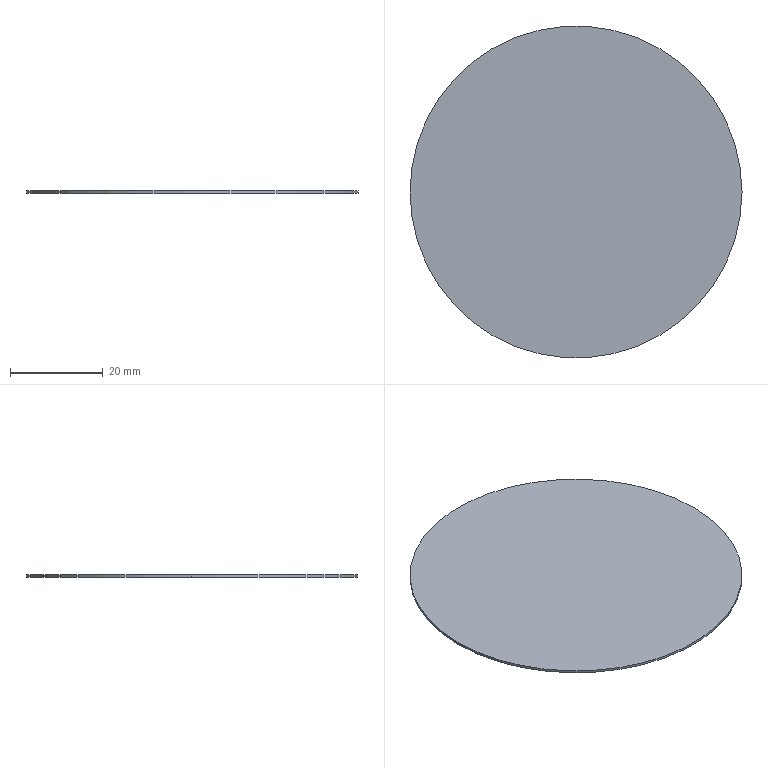Part | SolidWorks | features BaseBody 1 | 1 solid | 4 faces | box 71.5 x 71.5 x 0.5 mm | volume 2008 mm3 | cylinder 2 | plane 2 | commonest cylinder face diameters 71.5 x2
STEP:
#1=CARTESIAN_POINT('',(-50.25,-25.,21.3));
#2=VERTEX_POINT('',#1);
#3=CARTESIAN_POINT('',(-121.75,-25.,21.3));
#4=VERTEX_POINT('',#3);
#5=CARTESIAN_POINT('',(-86.,-25.,21.3));
#6=DIRECTION('',(0.,0.,1.));
#7=DIRECTION('',(1.,0.,0.));
#8=AXIS2_PLACEMENT_3D('',#5,#6,#7);
#9=CIRCLE('',#8,35.75);
#10=EDGE_CURVE('',#2,#4,#9,.T.);
#11=ORIENTED_EDGE('',*,*,#10,.T.);
#12=CARTESIAN_POINT('',(-121.75,-25.,21.8));
#13=VERTEX_POINT('',#12);
#14=CARTESIAN_POINT('',(-121.75,-25.,21.3));
#15=DIRECTION('',(0.,0.,1.));
#16=VECTOR('',#15,1000.);
#17=LINE('',#14,#16);
#18=EDGE_CURVE('',#4,#13,#17,.T.);
#19=ORIENTED_EDGE('',*,*,#18,.T.);
#20=CARTESIAN_POINT('',(-50.25,-25.,21.8));
#21=VERTEX_POINT('',#20);
#22=CARTESIAN_POINT('',(-86.,-25.,21.8));
#23=DIRECTION('',(0.,0.,-1.));
#24=DIRECTION('',(1.,0.,0.));
#25=AXIS2_PLACEMENT_3D('',#22,#23,#24);
#26=CIRCLE('',#25,35.75);
#27=EDGE_CURVE('',#13,#21,#26,.T.);
#28=ORIENTED_EDGE('',*,*,#27,.T.);
#29=CARTESIAN_POINT('',(-50.25,-25.,21.3));
#30=DIRECTION('',(0.,0.,1.));
#31=VECTOR('',#30,1000.);
#32=LINE('',#29,#31);
#33=EDGE_CURVE('',#2,#21,#32,.T.);
#34=ORIENTED_EDGE('',*,*,#33,.F.);
#35=EDGE_LOOP('',(#11,#19,#28,#34));
#36=FACE_OUTER_BOUND('',#35,.T.);
#37=CARTESIAN_POINT('',(-86.,-25.,21.3));
#38=DIRECTION('',(0.,0.,1.));
#39=DIRECTION('',(1.,0.,0.));
#40=AXIS2_PLACEMENT_3D('',#37,#38,#39);
#41=CYLINDRICAL_SURFACE('',#40,35.75);
#42=ADVANCED_FACE('',(#36),#41,.T.);
#43=CARTESIAN_POINT('',(-86.,-25.,21.8));
#44=DIRECTION('',(0.,0.,-1.));
#45=DIRECTION('',(1.,0.,0.));
#46=AXIS2_PLACEMENT_3D('',#43,#44,#45);
#47=CIRCLE('',#46,35.75);
#48=EDGE_CURVE('',#21,#13,#47,.T.);
#49=ORIENTED_EDGE('',*,*,#48,.F.);
#50=ORIENTED_EDGE('',*,*,#27,.F.);
#51=EDGE_LOOP('',(#49,#50));
#52=FACE_OUTER_BOUND('',#51,.T.);
#53=CARTESIAN_POINT('',(-86.,-25.,21.8));
#54=DIRECTION('',(0.,0.,1.));
#55=DIRECTION('',(1.,0.,0.));
#56=AXIS2_PLACEMENT_3D('',#53,#54,#55);
#57=PLANE('',#56);
#58=ADVANCED_FACE('',(#52),#57,.T.);
#59=ORIENTED_EDGE('',*,*,#10,.F.);
#60=CARTESIAN_POINT('',(-86.,-25.,21.3));
#61=DIRECTION('',(0.,0.,1.));
#62=DIRECTION('',(1.,0.,0.));
#63=AXIS2_PLACEMENT_3D('',#60,#61,#62);
#64=CIRCLE('',#63,35.75);
#65=EDGE_CURVE('',#4,#2,#64,.T.);
#66=ORIENTED_EDGE('',*,*,#65,.F.);
#67=EDGE_LOOP('',(#59,#66));
#68=FACE_OUTER_BOUND('',#67,.T.);
#69=CARTESIAN_POINT('',(-86.,-25.,21.3));
#70=DIRECTION('',(0.,0.,-1.));
#71=DIRECTION('',(-1.,0.,0.));
#72=AXIS2_PLACEMENT_3D('',#69,#70,#71);
#73=PLANE('',#72);
#74=ADVANCED_FACE('',(#68),#73,.T.);
#75=ORIENTED_EDGE('',*,*,#18,.F.);
#76=ORIENTED_EDGE('',*,*,#65,.T.);
#77=ORIENTED_EDGE('',*,*,#33,.T.);
#78=ORIENTED_EDGE('',*,*,#48,.T.);
#79=EDGE_LOOP('',(#75,#76,#77,#78));
#80=FACE_OUTER_BOUND('',#79,.T.);
#81=CARTESIAN_POINT('',(-86.,-25.,21.3));
#82=DIRECTION('',(0.,0.,1.));
#83=DIRECTION('',(1.,0.,0.));
#84=AXIS2_PLACEMENT_3D('',#81,#82,#83);
#85=CYLINDRICAL_SURFACE('',#84,35.75);
#86=ADVANCED_FACE('',(#80),#85,.T.);
#87=CLOSED_SHELL('',(#42,#58,#74,#86));
#88=MANIFOLD_SOLID_BREP('',#87);
#89=CARTESIAN_POINT('',(0.,0.,0.));
#90=DIRECTION('',(0.,0.,1.));
#91=DIRECTION('',(1.,0.,0.));
#92=AXIS2_PLACEMENT_3D('',#89,#90,#91);
#93=(LENGTH_UNIT()NAMED_UNIT(*)SI_UNIT(.MILLI.,.METRE.));
#94=UNCERTAINTY_MEASURE_WITH_UNIT(LENGTH_MEASURE(0.00001),#93,'','');
#95=(NAMED_UNIT(*)PLANE_ANGLE_UNIT()SI_UNIT($,.RADIAN.));
#96=(NAMED_UNIT(*)SI_UNIT($,.STERADIAN.)SOLID_ANGLE_UNIT());
#97=(GEOMETRIC_REPRESENTATION_CONTEXT(3)GLOBAL_UNCERTAINTY_ASSIGNED_CONTEXT((#94))GLOBAL_UNIT_ASSIGNED_CONTEXT((#93,#95,#96))REPRESENTATION_CONTEXT('',''));
#98=ADVANCED_BREP_SHAPE_REPRESENTATION('',(#88,#92),#97);